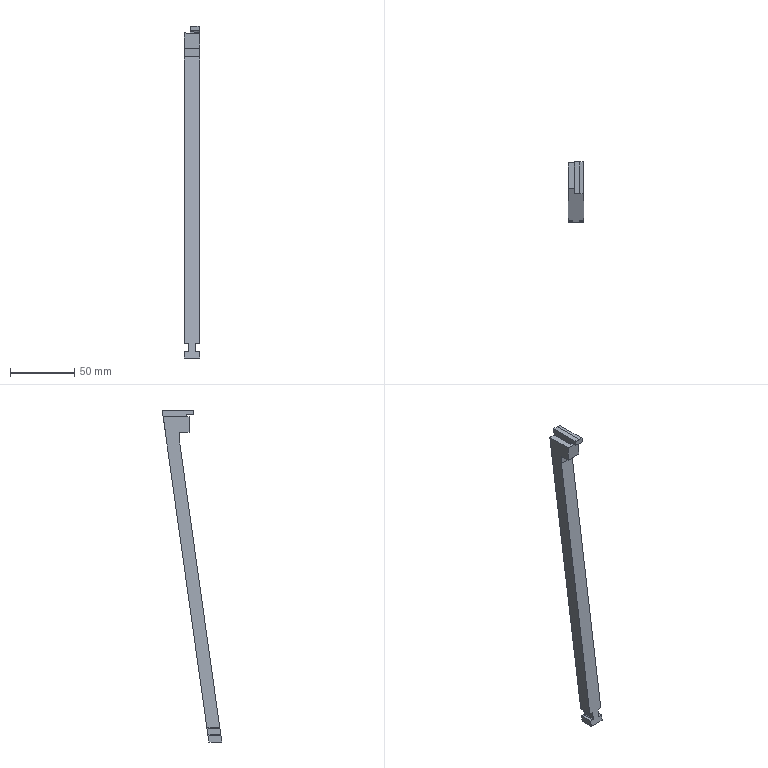Part | Creo | 1 solid | 102 faces | box 12 x 46.478 x 258.858 mm | volume 32486 mm3 | plane 59 | other 37 | cylinder 6 | commonest cylinder face diameters 1 x4 2 x1 26.509 x1